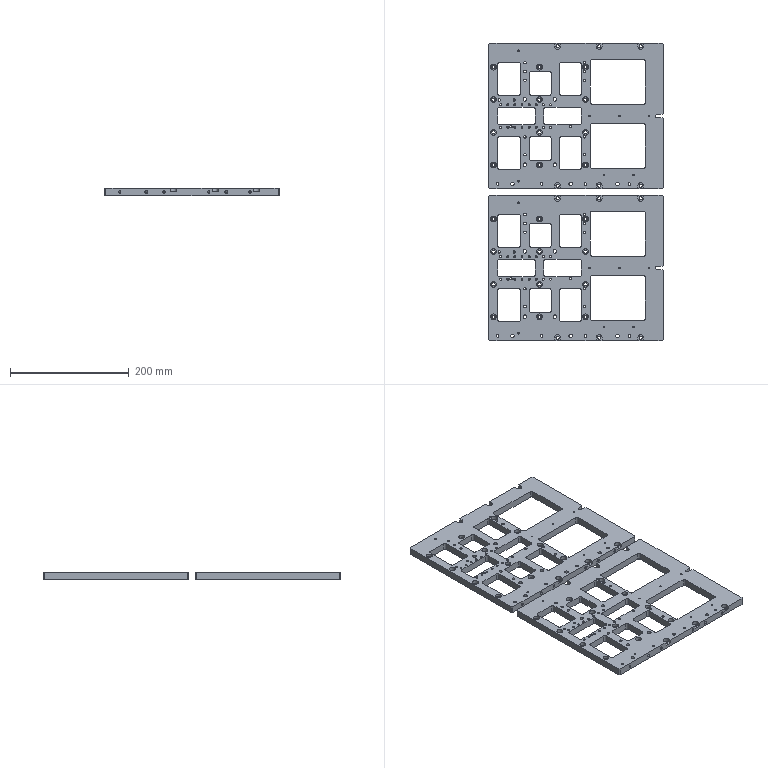NC program | NX | posted with a generic post | part box 294 x 501 x 12 mm
Whole program:
N10 G17 G21 G94 G90
(DRILLING_COPY_1_COPY_1_COPY , TOOL : D6A45)
N12 T22 M6
N14 G54
N16 G17 G0 G90 X77. Y0. B0. C0. S5000 M3
N18 G43 Z30. H22
N20 G94 G81 G98 Z-1. F250. R3.
N22 X-58.
N24 X122.
N26 X47.
N28 X-28.
N30 X-98.
N32 G80
N34 G0 X-98. Y0. Z30.
N36 M5
(DRILLING_COPY_1_COPY_COPY_COPY_COPY_1_COPY_COPY_1_COPY_COPY_1_COPY_2 , TOOL : )
N38 T21 M6
N40 G54
N42 G17 G0 G90 X122. Y0. B0. C0. S2000 M3
N44 G43 Z30. H21
N46 G94 G83 G98 Z-13.262 F150. Q2. R3.
N48 X47.
N50 X-28.
N52 X-98.
N54 X-58. Z-11.502
N56 X77.
N58 G80
N60 G0 X77. Y0. Z30.
N62 M5
(HOLE_MILLING_COPY_COPY_COPY_COPY , TOOL : D3)
N64 T13 M6
N66 G54
N68 G17 G0 G90 X-58. Y0. B0. C0. S7500 M3
N70 G43 Z30. H13
N72 Z0.5
N74 G94 G3 X-58.45 Y0.45 R0.45 F1000.
N76 X-58.9 Y0. R0.45
N78 X-58.9 Y0. Z0.2 I0.9 J0.
N80 X-58.9 Y0. Z-0.1 I0.9 J0.
N82 X-58.9 Y0. Z-0.4 I0.9 J0.
N84 X-58.9 Y0. Z-0.7 I0.9 J0.
N86 X-58.9 Y0. Z-1. I0.9 J0.
N88 X-58.9 Y0. Z-1.3 I0.9 J0.
N90 X-58.9 Y0. Z-1.6 I0.9 J0.
N92 X-58.9 Y0. Z-1.9 I0.9 J0.
N94 X-58.9 Y0. Z-2.2 I0.9 J0.
N96 X-58.9 Y0. Z-2.5 I0.9 J0.
N98 X-58.9 Y0. Z-2.8 I0.9 J0.
N100 X-58.9 Y0. Z-3.1 I0.9 J0.
N102 X-58.9 Y0. Z-3.4 I0.9 J0.
N104 X-58.9 Y0. Z-3.7 I0.9 J0.
N106 X-58.9 Y0. Z-4. I0.9 J0.
N108 X-58.9 Y0. Z-4.3 I0.9 J0.
N110 X-58.9 Y0. Z-4.6 I0.9 J0.
N112 X-58.9 Y0. Z-4.9 I0.9 J0.
N114 X-58.9 Y0. Z-5.2 I0.9 J0.
N116 X-58.9 Y0. Z-5.5 I0.9 J0.
N118 X-58.9 Y0. Z-5.8 I0.9 J0.
N120 X-58.9 Y0. Z-6.1 I0.9 J0.
N122 X-58.9 Y0. Z-6.4 I0.9 J0.
N124 X-58.9 Y0. Z-6.7 I0.9 J0.
N126 X-58.9 Y0. Z-7. I0.9 J0.
N128 X-58.9 Y0. Z-7.3 I0.9 J0.
N130 X-58.9 Y0. Z-7.6 I0.9 J0.
N132 X-58.9 Y0. Z-7.9 I0.9 J0.
N134 X-58.9 Y0. Z-8.2 I0.9 J0.
N136 X-58.9 Y0. Z-8.5 I0.9 J0.
N138 X-58.9 Y0. Z-8.8 I0.9 J0.
N140 X-58.9 Y0. Z-9.1 I0.9 J0.
N142 X-58.9 Y0. Z-9.4 I0.9 J0.
N144 X-58.9 Y0. Z-9.7 I0.9 J0.
N146 X-58.9 Y0. Z-10. I0.9 J0.
N148 X-58. Y-0.9 R0.9
N150 X-58.9 Y0. R-0.9
N152 X-58.45 Y-0.45 R0.45
N154 X-58. Y0. R0.45
N156 G0 Z30.
N158 X77.
N160 Z0.5
N162 G3 X76.55 Y0.45 R0.45
N164 X76.1 Y0. R0.45
N166 X76.1 Y0. Z0.2 I0.9 J0.
N168 X76.1 Y0. Z-0.1 I0.9 J0.
N170 X76.1 Y0. Z-0.4 I0.9 J0.
N172 X76.1 Y0. Z-0.7 I0.9 J0.
N174 X76.1 Y0. Z-1. I0.9 J0.
N176 X76.1 Y0. Z-1.3 I0.9 J0.
N178 X76.1 Y0. Z-1.6 I0.9 J0.
N180 X76.1 Y0. Z-1.9 I0.9 J0.
N182 X76.1 Y0. Z-2.2 I0.9 J0.
N184 X76.1 Y0. Z-2.5 I0.9 J0.
N186 X76.1 Y0. Z-2.8 I0.9 J0.
N188 X76.1 Y0. Z-3.1 I0.9 J0.
N190 X76.1 Y0. Z-3.4 I0.9 J0.
N192 X76.1 Y0. Z-3.7 I0.9 J0.
N194 X76.1 Y0. Z-4. I0.9 J0.
N196 X76.1 Y0. Z-4.3 I0.9 J0.
N198 X76.1 Y0. Z-4.6 I0.9 J0.
N200 X76.1 Y0. Z-4.9 I0.9 J0.
N202 X76.1 Y0. Z-5.2 I0.9 J0.
N204 X76.1 Y0. Z-5.5 I0.9 J0.
N206 X76.1 Y0. Z-5.8 I0.9 J0.
N208 X76.1 Y0. Z-6.1 I0.9 J0.
N210 X76.1 Y0. Z-6.4 I0.9 J0.
N212 X76.1 Y0. Z-6.7 I0.9 J0.
N214 X76.1 Y0. Z-7. I0.9 J0.
N216 X76.1 Y0. Z-7.3 I0.9 J0.
N218 X76.1 Y0. Z-7.6 I0.9 J0.
N220 X76.1 Y0. Z-7.9 I0.9 J0.
N222 X76.1 Y0. Z-8.2 I0.9 J0.
N224 X76.1 Y0. Z-8.5 I0.9 J0.
N226 X76.1 Y0. Z-8.8 I0.9 J0.
N228 X76.1 Y0. Z-9.1 I0.9 J0.
N230 X76.1 Y0. Z-9.4 I0.9 J0.
N232 X76.1 Y0. Z-9.7 I0.9 J0.
N234 X76.1 Y0. Z-10. I0.9 J0.
N236 X77. Y-0.9 R0.9
N238 X76.1 Y0. R-0.9
N240 X76.55 Y-0.45 R0.45
N242 X77. Y0. R0.45
N244 G0 Z30.
N246 M5
(刀补15_COPY , TOOL : D3)
N248 M6
N250 G54
N252 G17 G0 G90 X-58. Y0. B0. C0. S7500 M3
N254 G43 Z30. H13
N256 Z0.5
N258 G41 G94 G1 X-58.004 Y0.1 F1000. D13
N260 G3 X-58.95 Y0. R0.478
N262 X-58.95 Y0. Z-1.5 I0.95 J0.
N264 X-58.95 Y0. Z-3.5 I0.95 J0.
N266 X-58.95 Y0. Z-5.5 I0.95 J0.
N268 X-58.95 Y0. Z-7.5 I0.95 J0.
N270 X-58.95 Y0. Z-9.5 I0.95 J0.
N272 X-58. Y-0.95 Z-10. R0.95
N274 X-57.05 Y0. R0.95
N276 X-58. Y-0.95 R-0.95
N278 X-57.9 Y-0.004 R0.478
N280 G40
N282 G1 X-58. Y0.
N284 G0 Z30.
N286 X77.
N288 Z0.5
N290 G41 G1 X76.996 Y0.1
N292 G3 X76.05 Y0. R0.478
N294 X76.05 Y0. Z-1.5 I0.95 J0.
N296 X76.05 Y0. Z-3.5 I0.95 J0.
N298 X76.05 Y0. Z-5.5 I0.95 J0.
N300 X76.05 Y0. Z-7.5 I0.95 J0.
N302 X76.05 Y0. Z-9.5 I0.95 J0.
N304 X77. Y-0.95 Z-10. R0.95
N306 X77.95 Y0. R0.95
N308 X77. Y-0.95 R-0.95
N310 X77.1 Y-0.004 R0.478
N312 G40
N314 G1 X77. Y0.
N316 G0 Z30.
N318 M5
N320 M2